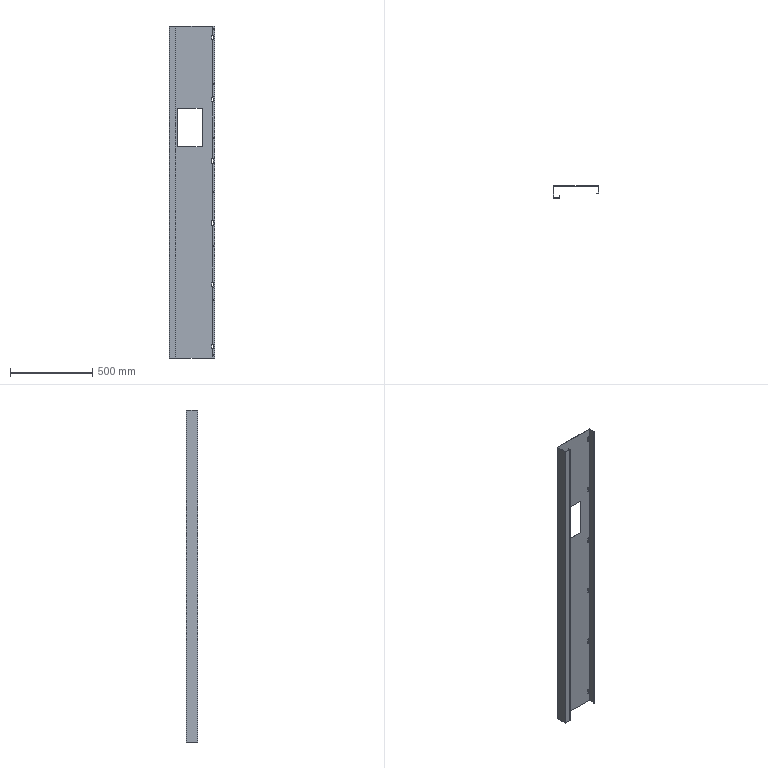Part | 1 solid | 132 faces | box 275 x 70 x 2016 mm | volume 1035938 mm3 | plane 76 | cylinder 56 | commonest cylinder face diameters 6.2 x28 9 x18 1 x5 3.4 x5